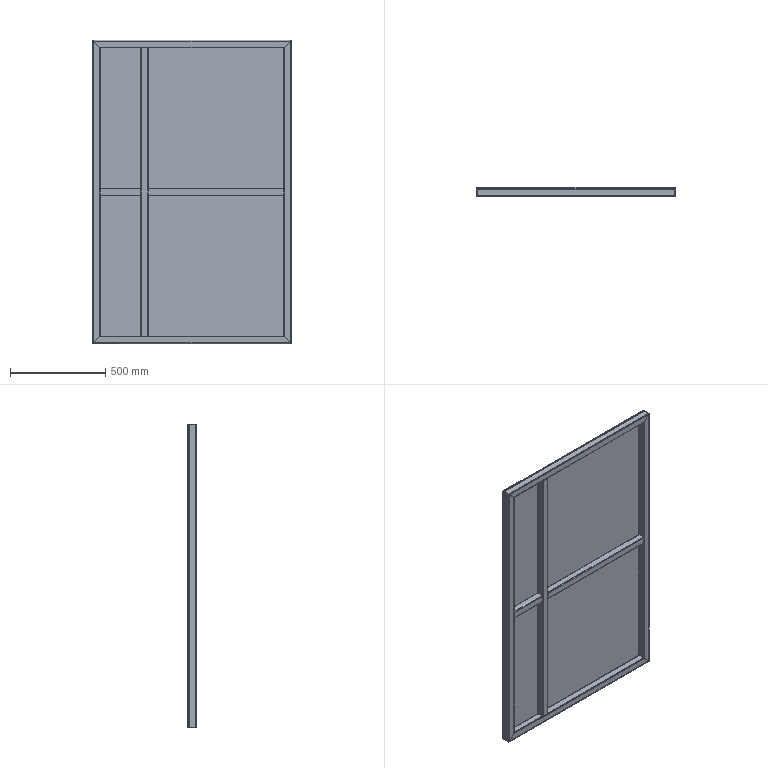Part | STEP file | Flip baffle_Default<Machined> | 8 solids | 132 faces | box 1040 x 45 x 1590 mm | volume 10479554 mm3 | plane 76 | cylinder 56 | commonest cylinder face diameters 4 x28 8 x28